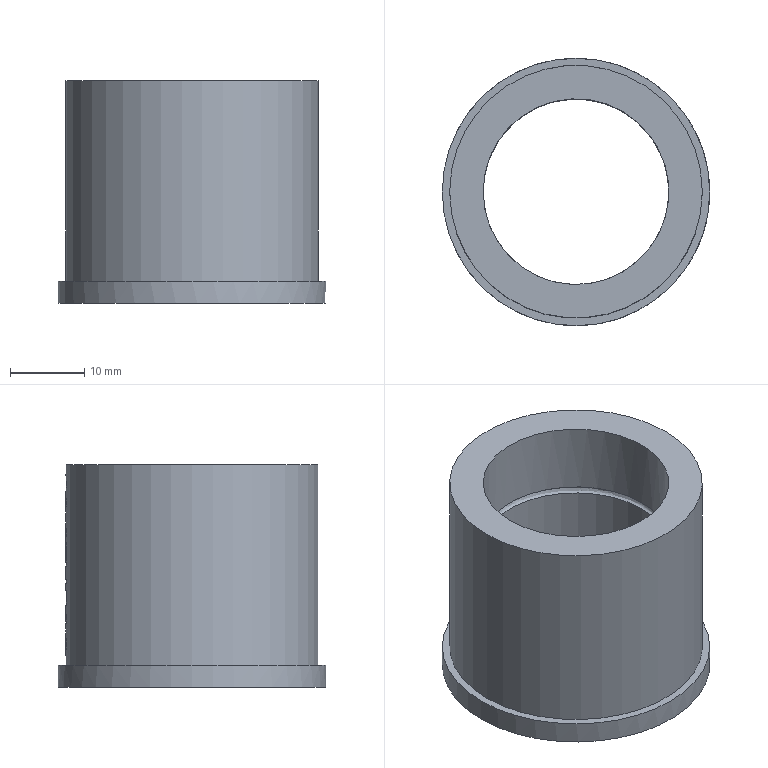Part | NX | features MI_SGBH_0847 2 | 1 solid | 144 faces | box 36 x 36 x 30 mm | volume 12736 mm3 | plane 77 | cylinder 65 | spline 2 | commonest cylinder face diameters 31.8 x9 25 x3 32 x3 2.113 x2 0.999 x1 1.035 x1